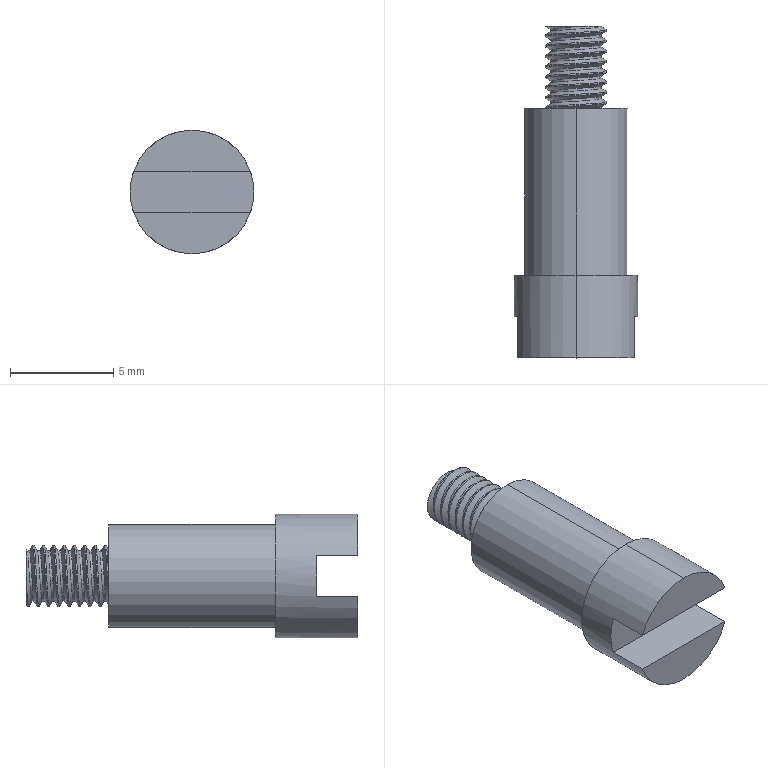Part | NX | features BREP 1 | 1 solid | 34 faces | box 6 x 16.1 x 6 mm | volume 271.92 mm3 | cylinder 23 | plane 9 | spline 2 | commonest cylinder face diameters 3 x18 5 x2 6 x2 2.459 x1